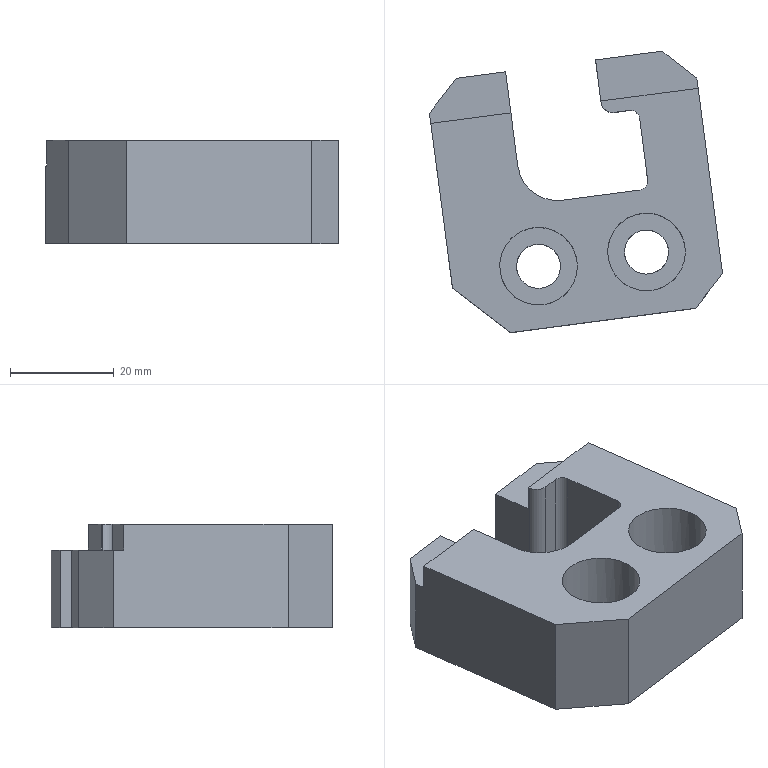Part | STEP file | gslz 2016.10.28-13_id534_x_t | 1 solid | 34 faces | box 56.515 x 54.271 x 20 mm | volume 31923 mm3 | plane 24 | cylinder 10 | commonest cylinder face diameters 3.5 x2 8.5 x2 11 x2 15 x2 4.5 x1 15.5 x1